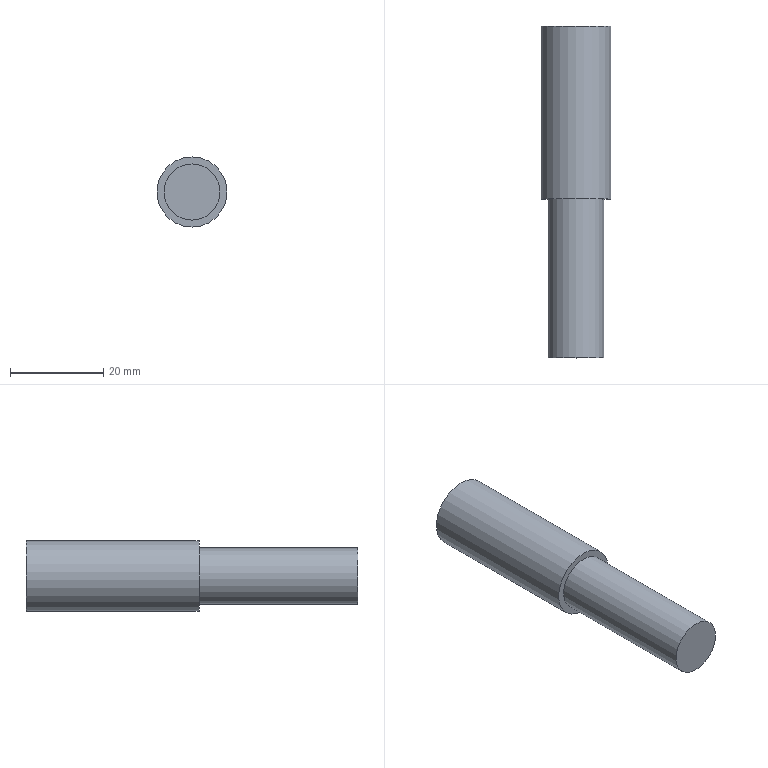Part | STEP file | chilunshuruzhou | 1 solid | 5 faces | box 15 x 71 x 15 mm | volume 10384 mm3 | plane 3 | cylinder 2 | commonest cylinder face diameters 12 x1 15 x1
STEP:
#1=CARTESIAN_POINT('',(0.,0.,0.));
#2=DIRECTION('',(0.,0.,1.));
#3=DIRECTION('',(1.,0.,0.));
#4=AXIS2_PLACEMENT_3D('',#1,#2,#3);
#5=CARTESIAN_POINT('',(0.,18.5,7.5));
#6=VERTEX_POINT('',#5);
#7=CARTESIAN_POINT('',(0.,18.5,0.));
#8=DIRECTION('',(0.,1.,0.));
#9=DIRECTION('',(0.,0.,1.));
#10=AXIS2_PLACEMENT_3D('',#7,#8,#9);
#11=CIRCLE('',#10,7.5);
#12=CARTESIAN_POINT('',(0.,18.5,0.));
#13=DIRECTION('',(0.,-1.,0.));
#14=DIRECTION('',(0.,0.,-1.));
#15=AXIS2_PLACEMENT_3D('',#12,#13,#14);
#16=CYLINDRICAL_SURFACE('',#15,7.5);
#17=CARTESIAN_POINT('',(9.425,0.));
#18=DIRECTION('',(-1.,0.));
#19=VECTOR('',#18,1.);
#20=LINE('',#17,#19);
#21=(GEOMETRIC_REPRESENTATION_CONTEXT(2)PARAMETRIC_REPRESENTATION_CONTEXT()REPRESENTATION_CONTEXT('',''));
#22=DEFINITIONAL_REPRESENTATION('',(#20),#21);
#23=PCURVE('',#16,#22);
#24=CARTESIAN_POINT('',(0.,18.5,0.));
#25=DIRECTION('',(0.,1.,0.));
#26=DIRECTION('',(0.,0.,1.));
#27=AXIS2_PLACEMENT_3D('',#24,#25,#26);
#28=PLANE('',#27);
#29=CARTESIAN_POINT('',(0.,0.));
#30=DIRECTION('',(1.,0.));
#31=AXIS2_PLACEMENT_2D('',#29,#30);
#32=CIRCLE('',#31,7.5);
#33=(GEOMETRIC_REPRESENTATION_CONTEXT(2)PARAMETRIC_REPRESENTATION_CONTEXT()REPRESENTATION_CONTEXT('',''));
#34=DEFINITIONAL_REPRESENTATION('',(#32),#33);
#35=PCURVE('',#28,#34);
#36=SURFACE_CURVE('',#11,(#23,#35),.PCURVE_S1.);
#37=EDGE_CURVE('',#6,#6,#36,.T.);
#38=ORIENTED_EDGE('',*,*,#37,.F.);
#39=CARTESIAN_POINT('',(0.,-18.5,7.5));
#40=VERTEX_POINT('',#39);
#41=CARTESIAN_POINT('',(0.,18.5,7.5));
#42=CARTESIAN_POINT('',(0.,-18.5,7.5));
#43=B_SPLINE_CURVE_WITH_KNOTS('',1,(#41,#42),.UNSPECIFIED.,.F.,.F.,(2,2),(0.,37.),.PIECEWISE_BEZIER_KNOTS.);
#44=CARTESIAN_POINT('',(9.425,0.));
#45=DIRECTION('',(0.,1.));
#46=VECTOR('',#45,1.);
#47=LINE('',#44,#46);
#48=(GEOMETRIC_REPRESENTATION_CONTEXT(2)PARAMETRIC_REPRESENTATION_CONTEXT()REPRESENTATION_CONTEXT('',''));
#49=DEFINITIONAL_REPRESENTATION('',(#47),#48);
#50=PCURVE('',#16,#49);
#51=CARTESIAN_POINT('',(3.142,0.));
#52=DIRECTION('',(0.,1.));
#53=VECTOR('',#52,1.);
#54=LINE('',#51,#53);
#55=(GEOMETRIC_REPRESENTATION_CONTEXT(2)PARAMETRIC_REPRESENTATION_CONTEXT()REPRESENTATION_CONTEXT('',''));
#56=DEFINITIONAL_REPRESENTATION('',(#54),#55);
#57=PCURVE('',#16,#56);
#58=SEAM_CURVE('',#43,(#50,#57),.PCURVE_S1.);
#59=EDGE_CURVE('',#6,#40,#58,.T.);
#60=ORIENTED_EDGE('',*,*,#59,.T.);
#61=CARTESIAN_POINT('',(0.,-18.5,0.));
#62=DIRECTION('',(0.,1.,0.));
#63=DIRECTION('',(0.,0.,1.));
#64=AXIS2_PLACEMENT_3D('',#61,#62,#63);
#65=CIRCLE('',#64,7.5);
#66=CARTESIAN_POINT('',(9.425,37.));
#67=DIRECTION('',(-1.,0.));
#68=VECTOR('',#67,1.);
#69=LINE('',#66,#68);
#70=(GEOMETRIC_REPRESENTATION_CONTEXT(2)PARAMETRIC_REPRESENTATION_CONTEXT()REPRESENTATION_CONTEXT('',''));
#71=DEFINITIONAL_REPRESENTATION('',(#69),#70);
#72=PCURVE('',#16,#71);
#73=CARTESIAN_POINT('',(0.,-18.5,0.));
#74=DIRECTION('',(0.,1.,0.));
#75=DIRECTION('',(0.,0.,1.));
#76=AXIS2_PLACEMENT_3D('',#73,#74,#75);
#77=PLANE('',#76);
#78=CARTESIAN_POINT('',(0.,0.));
#79=DIRECTION('',(1.,0.));
#80=AXIS2_PLACEMENT_2D('',#78,#79);
#81=CIRCLE('',#80,7.5);
#82=(GEOMETRIC_REPRESENTATION_CONTEXT(2)PARAMETRIC_REPRESENTATION_CONTEXT()REPRESENTATION_CONTEXT('',''));
#83=DEFINITIONAL_REPRESENTATION('',(#81),#82);
#84=PCURVE('',#77,#83);
#85=SURFACE_CURVE('',#65,(#72,#84),.PCURVE_S1.);
#86=EDGE_CURVE('',#40,#40,#85,.T.);
#87=ORIENTED_EDGE('',*,*,#86,.T.);
#88=ORIENTED_EDGE('',*,*,#59,.F.);
#89=EDGE_LOOP('',(#38,#60,#87,#88));
#90=FACE_BOUND('',#89,.T.);
#91=ADVANCED_FACE('',(#90),#16,.T.);
#92=ORIENTED_EDGE('',*,*,#37,.T.);
#93=EDGE_LOOP('',(#92));
#94=FACE_BOUND('',#93,.T.);
#95=ADVANCED_FACE('',(#94),#28,.T.);
#96=CARTESIAN_POINT('',(0.,-18.5,6.));
#97=VERTEX_POINT('',#96);
#98=CARTESIAN_POINT('',(0.,-18.5,0.));
#99=DIRECTION('',(0.,-1.,0.));
#100=DIRECTION('',(0.,0.,1.));
#101=AXIS2_PLACEMENT_3D('',#98,#99,#100);
#102=CIRCLE('',#101,6.);
#103=CARTESIAN_POINT('',(6.,0.));
#104=CARTESIAN_POINT('',(6.,-10.392));
#105=CARTESIAN_POINT('',(-3.,-5.196));
#106=CARTESIAN_POINT('',(-12.,0.));
#107=CARTESIAN_POINT('',(-3.,5.196));
#108=CARTESIAN_POINT('',(6.,10.392));
#109=CARTESIAN_POINT('',(6.,0.));
#110=(BOUNDED_CURVE()B_SPLINE_CURVE(2,(#103,#104,#105,#106,#107,#108,#109),.UNSPECIFIED.,.T.,.F.)B_SPLINE_CURVE_WITH_KNOTS((1,2,2,2,2,1),(-2.094,0.,2.094,4.189,6.283,8.378),.UNSPECIFIED.)CURVE()GEOMETRIC_REPRESENTATION_ITEM()RATIONAL_B_SPLINE_CURVE((1.,0.5,1.,0.5,1.,0.5,1.))REPRESENTATION_ITEM(''));
#111=(GEOMETRIC_REPRESENTATION_CONTEXT(2)PARAMETRIC_REPRESENTATION_CONTEXT()REPRESENTATION_CONTEXT('',''));
#112=DEFINITIONAL_REPRESENTATION('',(#110),#111);
#113=PCURVE('',#77,#112);
#114=CARTESIAN_POINT('',(0.,-52.5,0.));
#115=DIRECTION('',(0.,1.,0.));
#116=DIRECTION('',(0.,0.,1.));
#117=AXIS2_PLACEMENT_3D('',#114,#115,#116);
#118=CYLINDRICAL_SURFACE('',#117,6.);
#119=CARTESIAN_POINT('',(6.283,34.));
#120=DIRECTION('',(-1.,0.));
#121=VECTOR('',#120,1.);
#122=LINE('',#119,#121);
#123=(GEOMETRIC_REPRESENTATION_CONTEXT(2)PARAMETRIC_REPRESENTATION_CONTEXT()REPRESENTATION_CONTEXT('',''));
#124=DEFINITIONAL_REPRESENTATION('',(#122),#123);
#125=PCURVE('',#118,#124);
#126=SURFACE_CURVE('',#102,(#113,#125),.PCURVE_S1.);
#127=EDGE_CURVE('',#97,#97,#126,.T.);
#128=ORIENTED_EDGE('',*,*,#127,.F.);
#129=EDGE_LOOP('',(#128));
#130=FACE_BOUND('',#129,.T.);
#131=ORIENTED_EDGE('',*,*,#86,.F.);
#132=EDGE_LOOP('',(#131));
#133=FACE_BOUND('',#132,.T.);
#134=ADVANCED_FACE('',(#130,#133),#77,.F.);
#135=CARTESIAN_POINT('',(0.,-52.5,6.));
#136=VERTEX_POINT('',#135);
#137=CARTESIAN_POINT('',(0.,-52.5,-6.));
#138=VERTEX_POINT('',#137);
#139=CARTESIAN_POINT('',(0.,-52.5,0.));
#140=DIRECTION('',(0.,-1.,0.));
#141=DIRECTION('',(0.,0.,-1.));
#142=AXIS2_PLACEMENT_3D('',#139,#140,#141);
#143=CIRCLE('',#142,6.);
#144=CARTESIAN_POINT('',(9.425,0.));
#145=DIRECTION('',(-1.,0.));
#146=VECTOR('',#145,1.);
#147=LINE('',#144,#146);
#148=(GEOMETRIC_REPRESENTATION_CONTEXT(2)PARAMETRIC_REPRESENTATION_CONTEXT()REPRESENTATION_CONTEXT('',''));
#149=DEFINITIONAL_REPRESENTATION('',(#147),#148);
#150=PCURVE('',#118,#149);
#151=CARTESIAN_POINT('',(0.,-52.5,0.));
#152=DIRECTION('',(0.,-1.,0.));
#153=DIRECTION('',(0.,0.,-1.));
#154=AXIS2_PLACEMENT_3D('',#151,#152,#153);
#155=PLANE('',#154);
#156=CARTESIAN_POINT('',(0.,0.));
#157=DIRECTION('',(1.,0.));
#158=AXIS2_PLACEMENT_2D('',#156,#157);
#159=CIRCLE('',#158,6.);
#160=(GEOMETRIC_REPRESENTATION_CONTEXT(2)PARAMETRIC_REPRESENTATION_CONTEXT()REPRESENTATION_CONTEXT('',''));
#161=DEFINITIONAL_REPRESENTATION('',(#159),#160);
#162=PCURVE('',#155,#161);
#163=SURFACE_CURVE('',#143,(#150,#162),.PCURVE_S1.);
#164=EDGE_CURVE('',#136,#138,#163,.T.);
#165=ORIENTED_EDGE('',*,*,#164,.F.);
#166=CARTESIAN_POINT('',(0.,-52.5,6.));
#167=CARTESIAN_POINT('',(0.,-18.5,6.));
#168=B_SPLINE_CURVE_WITH_KNOTS('',1,(#166,#167),.UNSPECIFIED.,.F.,.F.,(2,2),(0.,34.),.PIECEWISE_BEZIER_KNOTS.);
#169=CARTESIAN_POINT('',(6.283,0.));
#170=DIRECTION('',(0.,1.));
#171=VECTOR('',#170,1.);
#172=LINE('',#169,#171);
#173=(GEOMETRIC_REPRESENTATION_CONTEXT(2)PARAMETRIC_REPRESENTATION_CONTEXT()REPRESENTATION_CONTEXT('',''));
#174=DEFINITIONAL_REPRESENTATION('',(#172),#173);
#175=PCURVE('',#118,#174);
#176=CARTESIAN_POINT('',(0.,0.));
#177=DIRECTION('',(0.,1.));
#178=VECTOR('',#177,1.);
#179=LINE('',#176,#178);
#180=(GEOMETRIC_REPRESENTATION_CONTEXT(2)PARAMETRIC_REPRESENTATION_CONTEXT()REPRESENTATION_CONTEXT('',''));
#181=DEFINITIONAL_REPRESENTATION('',(#179),#180);
#182=PCURVE('',#118,#181);
#183=SEAM_CURVE('',#168,(#175,#182),.PCURVE_S1.);
#184=EDGE_CURVE('',#136,#97,#183,.T.);
#185=ORIENTED_EDGE('',*,*,#184,.T.);
#186=ORIENTED_EDGE('',*,*,#127,.T.);
#187=ORIENTED_EDGE('',*,*,#184,.F.);
#188=CARTESIAN_POINT('',(0.,-52.5,0.));
#189=DIRECTION('',(0.,-1.,0.));
#190=DIRECTION('',(0.,0.,-1.));
#191=AXIS2_PLACEMENT_3D('',#188,#189,#190);
#192=CIRCLE('',#191,6.);
#193=CARTESIAN_POINT('',(3.142,0.));
#194=DIRECTION('',(-1.,0.));
#195=VECTOR('',#194,1.);
#196=LINE('',#193,#195);
#197=(GEOMETRIC_REPRESENTATION_CONTEXT(2)PARAMETRIC_REPRESENTATION_CONTEXT()REPRESENTATION_CONTEXT('',''));
#198=DEFINITIONAL_REPRESENTATION('',(#196),#197);
#199=PCURVE('',#118,#198);
#200=CARTESIAN_POINT('',(0.,0.));
#201=DIRECTION('',(1.,0.));
#202=AXIS2_PLACEMENT_2D('',#200,#201);
#203=CIRCLE('',#202,6.);
#204=(GEOMETRIC_REPRESENTATION_CONTEXT(2)PARAMETRIC_REPRESENTATION_CONTEXT()REPRESENTATION_CONTEXT('',''));
#205=DEFINITIONAL_REPRESENTATION('',(#203),#204);
#206=PCURVE('',#155,#205);
#207=SURFACE_CURVE('',#192,(#199,#206),.PCURVE_S1.);
#208=EDGE_CURVE('',#138,#136,#207,.T.);
#209=ORIENTED_EDGE('',*,*,#208,.F.);
#210=EDGE_LOOP('',(#165,#185,#186,#187,#209));
#211=FACE_BOUND('',#210,.T.);
#212=ADVANCED_FACE('',(#211),#118,.T.);
#213=ORIENTED_EDGE('',*,*,#208,.T.);
#214=ORIENTED_EDGE('',*,*,#164,.T.);
#215=EDGE_LOOP('',(#213,#214));
#216=FACE_BOUND('',#215,.T.);
#217=ADVANCED_FACE('',(#216),#155,.T.);
#218=CLOSED_SHELL('',(#91,#95,#134,#212,#217));
#219=MANIFOLD_SOLID_BREP('',#218);
#220=(LENGTH_UNIT()NAMED_UNIT(*)SI_UNIT(.MILLI.,.METRE.));
#221=UNCERTAINTY_MEASURE_WITH_UNIT(LENGTH_MEASURE(0.000005),#220,'','');
#222=(NAMED_UNIT(*)PLANE_ANGLE_UNIT()SI_UNIT($,.RADIAN.));
#223=(NAMED_UNIT(*)SI_UNIT($,.STERADIAN.)SOLID_ANGLE_UNIT());
#224=(GEOMETRIC_REPRESENTATION_CONTEXT(3)GLOBAL_UNCERTAINTY_ASSIGNED_CONTEXT((#221))GLOBAL_UNIT_ASSIGNED_CONTEXT((#220,#222,#223))REPRESENTATION_CONTEXT('',''));
#225=ADVANCED_BREP_SHAPE_REPRESENTATION('',(#4,#219),#224);